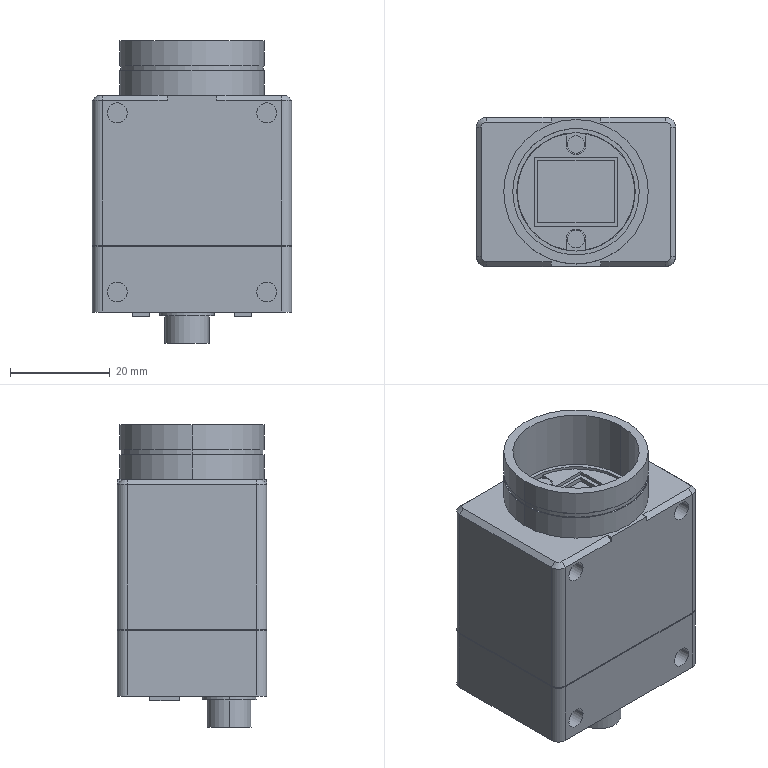Part | STEP file | camera-STC-MCS122BPOE.step.STEP [2] | 1 solid | 195 faces | box 40 x 30 x 60.8 mm | volume 51629 mm3 | plane 114 | cylinder 77 | cone 4 | commonest cylinder face diameters 4 x26 4.5 x8 4.9 x8 2 x4 3.5 x4 3.6 x4